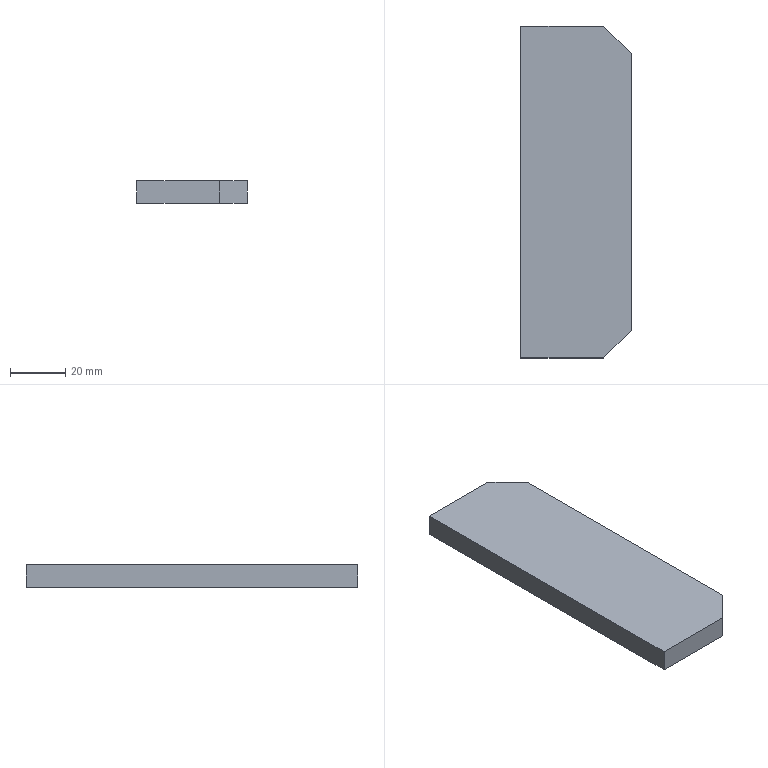Part | STEP file | 1 solid | 8 faces | box 40 x 120 x 8 mm | volume 37600 mm3 | plane 8
STEP:
#1=CARTESIAN_POINT('',(-20.,-60.,0.));
#2=VERTEX_POINT('',#1);
#3=CARTESIAN_POINT('',(-20.,-60.,8.));
#4=VERTEX_POINT('',#3);
#5=CARTESIAN_POINT('',(-20.,-60.,0.));
#6=DIRECTION('',(0.,0.,1.));
#7=VECTOR('',#6,1000.);
#8=LINE('',#5,#7);
#9=EDGE_CURVE('',#2,#4,#8,.T.);
#10=ORIENTED_EDGE('',*,*,#9,.T.);
#11=CARTESIAN_POINT('',(-20.,60.,8.));
#12=VERTEX_POINT('',#11);
#13=CARTESIAN_POINT('',(-20.,-60.,8.));
#14=DIRECTION('',(0.,1.,0.));
#15=VECTOR('',#14,1000.);
#16=LINE('',#13,#15);
#17=EDGE_CURVE('',#4,#12,#16,.T.);
#18=ORIENTED_EDGE('',*,*,#17,.T.);
#19=CARTESIAN_POINT('',(-20.,60.,0.));
#20=VERTEX_POINT('',#19);
#21=CARTESIAN_POINT('',(-20.,60.,0.));
#22=DIRECTION('',(0.,0.,1.));
#23=VECTOR('',#22,1000.);
#24=LINE('',#21,#23);
#25=EDGE_CURVE('',#20,#12,#24,.T.);
#26=ORIENTED_EDGE('',*,*,#25,.F.);
#27=CARTESIAN_POINT('',(-20.,-60.,0.));
#28=DIRECTION('',(0.,1.,0.));
#29=VECTOR('',#28,1000.);
#30=LINE('',#27,#29);
#31=EDGE_CURVE('',#2,#20,#30,.T.);
#32=ORIENTED_EDGE('',*,*,#31,.F.);
#33=EDGE_LOOP('',(#10,#18,#26,#32));
#34=FACE_OUTER_BOUND('',#33,.T.);
#35=CARTESIAN_POINT('',(-20.,-60.,8.));
#36=DIRECTION('',(1.,0.,0.));
#37=DIRECTION('',(0.,1.,0.));
#38=AXIS2_PLACEMENT_3D('',#35,#36,#37);
#39=PLANE('',#38);
#40=ADVANCED_FACE('',(#34),#39,.F.);
#41=CARTESIAN_POINT('',(10.,60.,0.));
#42=VERTEX_POINT('',#41);
#43=CARTESIAN_POINT('',(10.,60.,8.));
#44=VERTEX_POINT('',#43);
#45=CARTESIAN_POINT('',(10.,60.,0.));
#46=DIRECTION('',(0.,0.,1.));
#47=VECTOR('',#46,1000.);
#48=LINE('',#45,#47);
#49=EDGE_CURVE('',#42,#44,#48,.T.);
#50=ORIENTED_EDGE('',*,*,#49,.F.);
#51=CARTESIAN_POINT('',(-20.,60.,0.));
#52=DIRECTION('',(1.,0.,0.));
#53=VECTOR('',#52,1000.);
#54=LINE('',#51,#53);
#55=EDGE_CURVE('',#20,#42,#54,.T.);
#56=ORIENTED_EDGE('',*,*,#55,.F.);
#57=ORIENTED_EDGE('',*,*,#25,.T.);
#58=CARTESIAN_POINT('',(-20.,60.,8.));
#59=DIRECTION('',(1.,0.,0.));
#60=VECTOR('',#59,1000.);
#61=LINE('',#58,#60);
#62=EDGE_CURVE('',#12,#44,#61,.T.);
#63=ORIENTED_EDGE('',*,*,#62,.T.);
#64=EDGE_LOOP('',(#50,#56,#57,#63));
#65=FACE_OUTER_BOUND('',#64,.T.);
#66=CARTESIAN_POINT('',(-20.,60.,8.));
#67=DIRECTION('',(0.,-1.,0.));
#68=DIRECTION('',(0.,0.,-1.));
#69=AXIS2_PLACEMENT_3D('',#66,#67,#68);
#70=PLANE('',#69);
#71=ADVANCED_FACE('',(#65),#70,.F.);
#72=CARTESIAN_POINT('',(20.,50.,8.));
#73=VERTEX_POINT('',#72);
#74=CARTESIAN_POINT('',(20.,50.,0.));
#75=VERTEX_POINT('',#74);
#76=CARTESIAN_POINT('',(20.,50.,8.));
#77=DIRECTION('',(0.,0.,-1.));
#78=VECTOR('',#77,1000.);
#79=LINE('',#76,#78);
#80=EDGE_CURVE('',#73,#75,#79,.T.);
#81=ORIENTED_EDGE('',*,*,#80,.T.);
#82=CARTESIAN_POINT('',(10.,60.,0.));
#83=DIRECTION('',(0.7071,-0.7071,0.));
#84=VECTOR('',#83,1000.);
#85=LINE('',#82,#84);
#86=EDGE_CURVE('',#42,#75,#85,.T.);
#87=ORIENTED_EDGE('',*,*,#86,.F.);
#88=ORIENTED_EDGE('',*,*,#49,.T.);
#89=CARTESIAN_POINT('',(20.,50.,8.));
#90=DIRECTION('',(-0.7071,0.7071,0.));
#91=VECTOR('',#90,1000.);
#92=LINE('',#89,#91);
#93=EDGE_CURVE('',#73,#44,#92,.T.);
#94=ORIENTED_EDGE('',*,*,#93,.F.);
#95=EDGE_LOOP('',(#81,#87,#88,#94));
#96=FACE_OUTER_BOUND('',#95,.T.);
#97=CARTESIAN_POINT('',(10.,60.,8.));
#98=DIRECTION('',(-0.7071,-0.7071,0.));
#99=DIRECTION('',(-0.7071,0.7071,0.));
#100=AXIS2_PLACEMENT_3D('',#97,#98,#99);
#101=PLANE('',#100);
#102=ADVANCED_FACE('',(#96),#101,.F.);
#103=CARTESIAN_POINT('',(20.,-50.,0.));
#104=VERTEX_POINT('',#103);
#105=CARTESIAN_POINT('',(20.,-50.,8.));
#106=VERTEX_POINT('',#105);
#107=CARTESIAN_POINT('',(20.,-50.,0.));
#108=DIRECTION('',(0.,0.,1.));
#109=VECTOR('',#108,1000.);
#110=LINE('',#107,#109);
#111=EDGE_CURVE('',#104,#106,#110,.T.);
#112=ORIENTED_EDGE('',*,*,#111,.F.);
#113=CARTESIAN_POINT('',(20.,50.,0.));
#114=DIRECTION('',(0.,-1.,0.));
#115=VECTOR('',#114,1000.);
#116=LINE('',#113,#115);
#117=EDGE_CURVE('',#75,#104,#116,.T.);
#118=ORIENTED_EDGE('',*,*,#117,.F.);
#119=ORIENTED_EDGE('',*,*,#80,.F.);
#120=CARTESIAN_POINT('',(20.,50.,8.));
#121=DIRECTION('',(0.,-1.,0.));
#122=VECTOR('',#121,1000.);
#123=LINE('',#120,#122);
#124=EDGE_CURVE('',#73,#106,#123,.T.);
#125=ORIENTED_EDGE('',*,*,#124,.T.);
#126=EDGE_LOOP('',(#112,#118,#119,#125));
#127=FACE_OUTER_BOUND('',#126,.T.);
#128=CARTESIAN_POINT('',(20.,-60.,8.));
#129=DIRECTION('',(-1.,0.,0.));
#130=DIRECTION('',(0.,0.,1.));
#131=AXIS2_PLACEMENT_3D('',#128,#129,#130);
#132=PLANE('',#131);
#133=ADVANCED_FACE('',(#127),#132,.F.);
#134=CARTESIAN_POINT('',(10.,-60.,0.));
#135=VERTEX_POINT('',#134);
#136=CARTESIAN_POINT('',(20.,-50.,0.));
#137=DIRECTION('',(-0.7071,-0.7071,0.));
#138=VECTOR('',#137,1000.);
#139=LINE('',#136,#138);
#140=EDGE_CURVE('',#104,#135,#139,.T.);
#141=ORIENTED_EDGE('',*,*,#140,.T.);
#142=CARTESIAN_POINT('',(10.,-60.,0.));
#143=DIRECTION('',(-1.,0.,0.));
#144=VECTOR('',#143,1000.);
#145=LINE('',#142,#144);
#146=EDGE_CURVE('',#135,#2,#145,.T.);
#147=ORIENTED_EDGE('',*,*,#146,.T.);
#148=ORIENTED_EDGE('',*,*,#31,.T.);
#149=ORIENTED_EDGE('',*,*,#55,.T.);
#150=ORIENTED_EDGE('',*,*,#86,.T.);
#151=ORIENTED_EDGE('',*,*,#117,.T.);
#152=EDGE_LOOP('',(#141,#147,#148,#149,#150,#151));
#153=FACE_OUTER_BOUND('',#152,.T.);
#154=CARTESIAN_POINT('',(0.,0.,0.));
#155=DIRECTION('',(0.,0.,-1.));
#156=DIRECTION('',(0.,-1.,0.));
#157=AXIS2_PLACEMENT_3D('',#154,#155,#156);
#158=PLANE('',#157);
#159=ADVANCED_FACE('',(#153),#158,.T.);
#160=CARTESIAN_POINT('',(10.,-60.,8.));
#161=VERTEX_POINT('',#160);
#162=CARTESIAN_POINT('',(10.,-60.,8.));
#163=DIRECTION('',(0.,0.,-1.));
#164=VECTOR('',#163,1000.);
#165=LINE('',#162,#164);
#166=EDGE_CURVE('',#161,#135,#165,.T.);
#167=ORIENTED_EDGE('',*,*,#166,.F.);
#168=CARTESIAN_POINT('',(10.,-60.,8.));
#169=DIRECTION('',(-1.,0.,0.));
#170=VECTOR('',#169,1000.);
#171=LINE('',#168,#170);
#172=EDGE_CURVE('',#161,#4,#171,.T.);
#173=ORIENTED_EDGE('',*,*,#172,.T.);
#174=ORIENTED_EDGE('',*,*,#9,.F.);
#175=ORIENTED_EDGE('',*,*,#146,.F.);
#176=EDGE_LOOP('',(#167,#173,#174,#175));
#177=FACE_OUTER_BOUND('',#176,.T.);
#178=CARTESIAN_POINT('',(-20.,-60.,8.));
#179=DIRECTION('',(0.,1.,0.));
#180=DIRECTION('',(1.,0.,0.));
#181=AXIS2_PLACEMENT_3D('',#178,#179,#180);
#182=PLANE('',#181);
#183=ADVANCED_FACE('',(#177),#182,.F.);
#184=CARTESIAN_POINT('',(10.,-60.,8.));
#185=DIRECTION('',(0.7071,0.7071,0.));
#186=VECTOR('',#185,1000.);
#187=LINE('',#184,#186);
#188=EDGE_CURVE('',#161,#106,#187,.T.);
#189=ORIENTED_EDGE('',*,*,#188,.T.);
#190=ORIENTED_EDGE('',*,*,#124,.F.);
#191=ORIENTED_EDGE('',*,*,#93,.T.);
#192=ORIENTED_EDGE('',*,*,#62,.F.);
#193=ORIENTED_EDGE('',*,*,#17,.F.);
#194=ORIENTED_EDGE('',*,*,#172,.F.);
#195=EDGE_LOOP('',(#189,#190,#191,#192,#193,#194));
#196=FACE_OUTER_BOUND('',#195,.T.);
#197=CARTESIAN_POINT('',(0.,0.,8.));
#198=DIRECTION('',(0.,0.,-1.));
#199=DIRECTION('',(0.,-1.,0.));
#200=AXIS2_PLACEMENT_3D('',#197,#198,#199);
#201=PLANE('',#200);
#202=ADVANCED_FACE('',(#196),#201,.F.);
#203=ORIENTED_EDGE('',*,*,#166,.T.);
#204=ORIENTED_EDGE('',*,*,#140,.F.);
#205=ORIENTED_EDGE('',*,*,#111,.T.);
#206=ORIENTED_EDGE('',*,*,#188,.F.);
#207=EDGE_LOOP('',(#203,#204,#205,#206));
#208=FACE_OUTER_BOUND('',#207,.T.);
#209=CARTESIAN_POINT('',(20.,-50.,8.));
#210=DIRECTION('',(-0.7071,0.7071,0.));
#211=DIRECTION('',(0.,0.,1.));
#212=AXIS2_PLACEMENT_3D('',#209,#210,#211);
#213=PLANE('',#212);
#214=ADVANCED_FACE('',(#208),#213,.F.);
#215=CLOSED_SHELL('',(#40,#71,#102,#133,#159,#183,#202,#214));
#216=MANIFOLD_SOLID_BREP('',#215);
#217=CARTESIAN_POINT('',(0.,0.,0.));
#218=DIRECTION('',(0.,0.,1.));
#219=DIRECTION('',(1.,0.,0.));
#220=AXIS2_PLACEMENT_3D('',#217,#218,#219);
#221=(LENGTH_UNIT()NAMED_UNIT(*)SI_UNIT(.MILLI.,.METRE.));
#222=UNCERTAINTY_MEASURE_WITH_UNIT(LENGTH_MEASURE(0.00001),#221,'','');
#223=(NAMED_UNIT(*)PLANE_ANGLE_UNIT()SI_UNIT($,.RADIAN.));
#224=(NAMED_UNIT(*)SI_UNIT($,.STERADIAN.)SOLID_ANGLE_UNIT());
#225=(GEOMETRIC_REPRESENTATION_CONTEXT(3)GLOBAL_UNCERTAINTY_ASSIGNED_CONTEXT((#222))GLOBAL_UNIT_ASSIGNED_CONTEXT((#221,#223,#224))REPRESENTATION_CONTEXT('',''));
#226=ADVANCED_BREP_SHAPE_REPRESENTATION('',(#216,#220),#225);